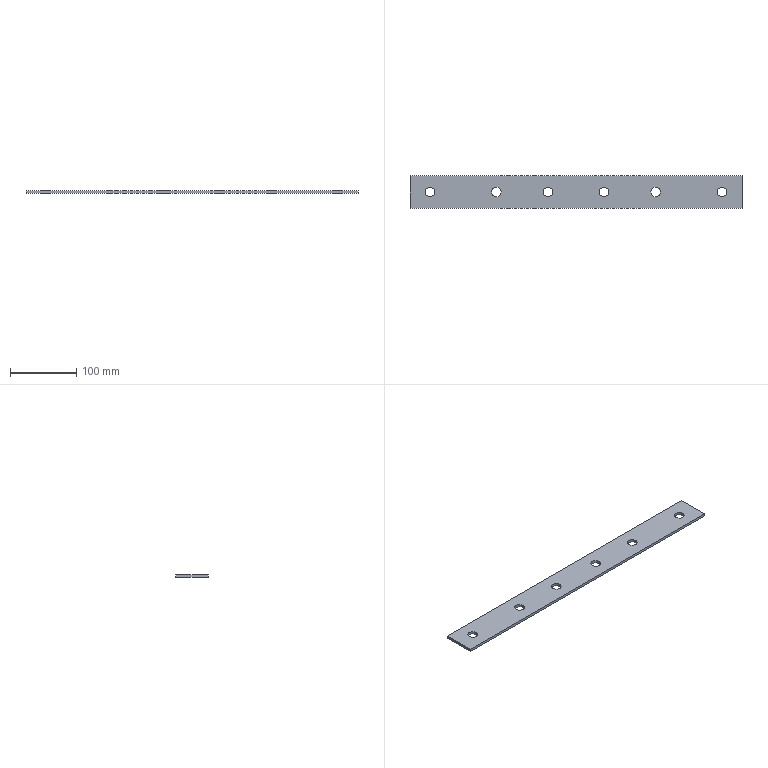Part | SolidWorks | features FlatPattern 1, ICE 1, MirrorPattern 1, SMBaseFlange 1, SheetMetal 1 | 1 solid | 18 faces | box 500 x 49 x 4 mm | volume 94037 mm3 | cylinder 12 | plane 6 | commonest cylinder face diameters 14.5 x12
STEP:
#1=CARTESIAN_POINT('',(-34.75,0.,-4.));
#2=VERTEX_POINT('',#1);
#3=CARTESIAN_POINT('',(-49.25,0.,-4.));
#4=VERTEX_POINT('',#3);
#5=CARTESIAN_POINT('',(-42.,0.,-4.));
#6=DIRECTION('',(0.,0.,-1.));
#7=DIRECTION('',(-1.,0.,0.));
#8=AXIS2_PLACEMENT_3D('',#5,#6,#7);
#9=CIRCLE('',#8,7.25);
#10=EDGE_CURVE('',#2,#4,#9,.T.);
#11=ORIENTED_EDGE('',*,*,#10,.T.);
#12=CARTESIAN_POINT('',(-49.25,0.,0.));
#13=VERTEX_POINT('',#12);
#14=CARTESIAN_POINT('',(-49.25,0.,-4.));
#15=DIRECTION('',(0.,0.,1.));
#16=VECTOR('',#15,1000.);
#17=LINE('',#14,#16);
#18=EDGE_CURVE('',#4,#13,#17,.T.);
#19=ORIENTED_EDGE('',*,*,#18,.T.);
#20=CARTESIAN_POINT('',(-34.75,0.,0.));
#21=VERTEX_POINT('',#20);
#22=CARTESIAN_POINT('',(-42.,0.,0.));
#23=DIRECTION('',(0.,0.,-1.));
#24=DIRECTION('',(1.,0.,0.));
#25=AXIS2_PLACEMENT_3D('',#22,#23,#24);
#26=CIRCLE('',#25,7.25);
#27=EDGE_CURVE('',#21,#13,#26,.T.);
#28=ORIENTED_EDGE('',*,*,#27,.F.);
#29=CARTESIAN_POINT('',(-34.75,0.,-4.));
#30=DIRECTION('',(0.,0.,1.));
#31=VECTOR('',#30,1000.);
#32=LINE('',#29,#31);
#33=EDGE_CURVE('',#2,#21,#32,.T.);
#34=ORIENTED_EDGE('',*,*,#33,.F.);
#35=EDGE_LOOP('',(#11,#19,#28,#34));
#36=FACE_OUTER_BOUND('',#35,.T.);
#37=CARTESIAN_POINT('',(-42.,0.,-4.));
#38=DIRECTION('',(0.,0.,1.));
#39=DIRECTION('',(1.,0.,0.));
#40=AXIS2_PLACEMENT_3D('',#37,#38,#39);
#41=CYLINDRICAL_SURFACE('',#40,7.25);
#42=ADVANCED_FACE('',(#36),#41,.F.);
#43=CARTESIAN_POINT('',(-112.75,0.,-4.));
#44=VERTEX_POINT('',#43);
#45=CARTESIAN_POINT('',(-127.25,0.,-4.));
#46=VERTEX_POINT('',#45);
#47=CARTESIAN_POINT('',(-120.,0.,-4.));
#48=DIRECTION('',(0.,0.,-1.));
#49=DIRECTION('',(-1.,0.,0.));
#50=AXIS2_PLACEMENT_3D('',#47,#48,#49);
#51=CIRCLE('',#50,7.25);
#52=EDGE_CURVE('',#44,#46,#51,.T.);
#53=ORIENTED_EDGE('',*,*,#52,.T.);
#54=CARTESIAN_POINT('',(-127.25,0.,0.));
#55=VERTEX_POINT('',#54);
#56=CARTESIAN_POINT('',(-127.25,0.,-4.));
#57=DIRECTION('',(0.,0.,1.));
#58=VECTOR('',#57,1000.);
#59=LINE('',#56,#58);
#60=EDGE_CURVE('',#46,#55,#59,.T.);
#61=ORIENTED_EDGE('',*,*,#60,.T.);
#62=CARTESIAN_POINT('',(-112.75,0.,0.));
#63=VERTEX_POINT('',#62);
#64=CARTESIAN_POINT('',(-120.,0.,0.));
#65=DIRECTION('',(0.,0.,-1.));
#66=DIRECTION('',(1.,0.,0.));
#67=AXIS2_PLACEMENT_3D('',#64,#65,#66);
#68=CIRCLE('',#67,7.25);
#69=EDGE_CURVE('',#63,#55,#68,.T.);
#70=ORIENTED_EDGE('',*,*,#69,.F.);
#71=CARTESIAN_POINT('',(-112.75,0.,-4.));
#72=DIRECTION('',(0.,0.,1.));
#73=VECTOR('',#72,1000.);
#74=LINE('',#71,#73);
#75=EDGE_CURVE('',#44,#63,#74,.T.);
#76=ORIENTED_EDGE('',*,*,#75,.F.);
#77=EDGE_LOOP('',(#53,#61,#70,#76));
#78=FACE_OUTER_BOUND('',#77,.T.);
#79=CARTESIAN_POINT('',(-120.,0.,-4.));
#80=DIRECTION('',(0.,0.,1.));
#81=DIRECTION('',(1.,0.,0.));
#82=AXIS2_PLACEMENT_3D('',#79,#80,#81);
#83=CYLINDRICAL_SURFACE('',#82,7.25);
#84=ADVANCED_FACE('',(#78),#83,.F.);
#85=CARTESIAN_POINT('',(-212.75,0.,-4.));
#86=VERTEX_POINT('',#85);
#87=CARTESIAN_POINT('',(-227.25,0.,-4.));
#88=VERTEX_POINT('',#87);
#89=CARTESIAN_POINT('',(-220.,0.,-4.));
#90=DIRECTION('',(0.,0.,-1.));
#91=DIRECTION('',(-1.,0.,0.));
#92=AXIS2_PLACEMENT_3D('',#89,#90,#91);
#93=CIRCLE('',#92,7.25);
#94=EDGE_CURVE('',#86,#88,#93,.T.);
#95=ORIENTED_EDGE('',*,*,#94,.T.);
#96=CARTESIAN_POINT('',(-227.25,0.,0.));
#97=VERTEX_POINT('',#96);
#98=CARTESIAN_POINT('',(-227.25,0.,-4.));
#99=DIRECTION('',(0.,0.,1.));
#100=VECTOR('',#99,1000.);
#101=LINE('',#98,#100);
#102=EDGE_CURVE('',#88,#97,#101,.T.);
#103=ORIENTED_EDGE('',*,*,#102,.T.);
#104=CARTESIAN_POINT('',(-212.75,0.,0.));
#105=VERTEX_POINT('',#104);
#106=CARTESIAN_POINT('',(-220.,0.,0.));
#107=DIRECTION('',(0.,0.,-1.));
#108=DIRECTION('',(1.,0.,0.));
#109=AXIS2_PLACEMENT_3D('',#106,#107,#108);
#110=CIRCLE('',#109,7.25);
#111=EDGE_CURVE('',#105,#97,#110,.T.);
#112=ORIENTED_EDGE('',*,*,#111,.F.);
#113=CARTESIAN_POINT('',(-212.75,0.,-4.));
#114=DIRECTION('',(0.,0.,1.));
#115=VECTOR('',#114,1000.);
#116=LINE('',#113,#115);
#117=EDGE_CURVE('',#86,#105,#116,.T.);
#118=ORIENTED_EDGE('',*,*,#117,.F.);
#119=EDGE_LOOP('',(#95,#103,#112,#118));
#120=FACE_OUTER_BOUND('',#119,.T.);
#121=CARTESIAN_POINT('',(-220.,0.,-4.));
#122=DIRECTION('',(0.,0.,1.));
#123=DIRECTION('',(1.,0.,0.));
#124=AXIS2_PLACEMENT_3D('',#121,#122,#123);
#125=CYLINDRICAL_SURFACE('',#124,7.25);
#126=ADVANCED_FACE('',(#120),#125,.F.);
#127=CARTESIAN_POINT('',(34.75,0.,-4.));
#128=VERTEX_POINT('',#127);
#129=CARTESIAN_POINT('',(49.25,0.,-4.));
#130=VERTEX_POINT('',#129);
#131=CARTESIAN_POINT('',(42.,0.,-4.));
#132=DIRECTION('',(0.,0.,1.));
#133=DIRECTION('',(1.,0.,0.));
#134=AXIS2_PLACEMENT_3D('',#131,#132,#133);
#135=CIRCLE('',#134,7.25);
#136=EDGE_CURVE('',#128,#130,#135,.T.);
#137=ORIENTED_EDGE('',*,*,#136,.F.);
#138=CARTESIAN_POINT('',(34.75,0.,0.));
#139=VERTEX_POINT('',#138);
#140=CARTESIAN_POINT('',(34.75,0.,-4.));
#141=DIRECTION('',(0.,0.,1.));
#142=VECTOR('',#141,1000.);
#143=LINE('',#140,#142);
#144=EDGE_CURVE('',#128,#139,#143,.T.);
#145=ORIENTED_EDGE('',*,*,#144,.T.);
#146=CARTESIAN_POINT('',(49.25,0.,0.));
#147=VERTEX_POINT('',#146);
#148=CARTESIAN_POINT('',(42.,0.,0.));
#149=DIRECTION('',(0.,0.,1.));
#150=DIRECTION('',(1.,0.,0.));
#151=AXIS2_PLACEMENT_3D('',#148,#149,#150);
#152=CIRCLE('',#151,7.25);
#153=EDGE_CURVE('',#139,#147,#152,.T.);
#154=ORIENTED_EDGE('',*,*,#153,.T.);
#155=CARTESIAN_POINT('',(49.25,0.,-4.));
#156=DIRECTION('',(0.,0.,1.));
#157=VECTOR('',#156,1000.);
#158=LINE('',#155,#157);
#159=EDGE_CURVE('',#130,#147,#158,.T.);
#160=ORIENTED_EDGE('',*,*,#159,.F.);
#161=EDGE_LOOP('',(#137,#145,#154,#160));
#162=FACE_OUTER_BOUND('',#161,.T.);
#163=CARTESIAN_POINT('',(42.,0.,-4.));
#164=DIRECTION('',(0.,0.,1.));
#165=DIRECTION('',(1.,0.,0.));
#166=AXIS2_PLACEMENT_3D('',#163,#164,#165);
#167=CYLINDRICAL_SURFACE('',#166,7.25);
#168=ADVANCED_FACE('',(#162),#167,.F.);
#169=CARTESIAN_POINT('',(112.75,0.,-4.));
#170=VERTEX_POINT('',#169);
#171=CARTESIAN_POINT('',(127.25,0.,-4.));
#172=VERTEX_POINT('',#171);
#173=CARTESIAN_POINT('',(120.,0.,-4.));
#174=DIRECTION('',(0.,0.,1.));
#175=DIRECTION('',(1.,0.,0.));
#176=AXIS2_PLACEMENT_3D('',#173,#174,#175);
#177=CIRCLE('',#176,7.25);
#178=EDGE_CURVE('',#170,#172,#177,.T.);
#179=ORIENTED_EDGE('',*,*,#178,.F.);
#180=CARTESIAN_POINT('',(112.75,0.,0.));
#181=VERTEX_POINT('',#180);
#182=CARTESIAN_POINT('',(112.75,0.,-4.));
#183=DIRECTION('',(0.,0.,1.));
#184=VECTOR('',#183,1000.);
#185=LINE('',#182,#184);
#186=EDGE_CURVE('',#170,#181,#185,.T.);
#187=ORIENTED_EDGE('',*,*,#186,.T.);
#188=CARTESIAN_POINT('',(127.25,0.,0.));
#189=VERTEX_POINT('',#188);
#190=CARTESIAN_POINT('',(120.,0.,0.));
#191=DIRECTION('',(0.,0.,1.));
#192=DIRECTION('',(1.,0.,0.));
#193=AXIS2_PLACEMENT_3D('',#190,#191,#192);
#194=CIRCLE('',#193,7.25);
#195=EDGE_CURVE('',#181,#189,#194,.T.);
#196=ORIENTED_EDGE('',*,*,#195,.T.);
#197=CARTESIAN_POINT('',(127.25,0.,-4.));
#198=DIRECTION('',(0.,0.,1.));
#199=VECTOR('',#198,1000.);
#200=LINE('',#197,#199);
#201=EDGE_CURVE('',#172,#189,#200,.T.);
#202=ORIENTED_EDGE('',*,*,#201,.F.);
#203=EDGE_LOOP('',(#179,#187,#196,#202));
#204=FACE_OUTER_BOUND('',#203,.T.);
#205=CARTESIAN_POINT('',(120.,0.,-4.));
#206=DIRECTION('',(0.,0.,1.));
#207=DIRECTION('',(1.,0.,0.));
#208=AXIS2_PLACEMENT_3D('',#205,#206,#207);
#209=CYLINDRICAL_SURFACE('',#208,7.25);
#210=ADVANCED_FACE('',(#204),#209,.F.);
#211=CARTESIAN_POINT('',(212.75,0.,-4.));
#212=VERTEX_POINT('',#211);
#213=CARTESIAN_POINT('',(227.25,0.,-4.));
#214=VERTEX_POINT('',#213);
#215=CARTESIAN_POINT('',(220.,0.,-4.));
#216=DIRECTION('',(0.,0.,1.));
#217=DIRECTION('',(1.,0.,0.));
#218=AXIS2_PLACEMENT_3D('',#215,#216,#217);
#219=CIRCLE('',#218,7.25);
#220=EDGE_CURVE('',#212,#214,#219,.T.);
#221=ORIENTED_EDGE('',*,*,#220,.F.);
#222=CARTESIAN_POINT('',(212.75,0.,0.));
#223=VERTEX_POINT('',#222);
#224=CARTESIAN_POINT('',(212.75,0.,-4.));
#225=DIRECTION('',(0.,0.,1.));
#226=VECTOR('',#225,1000.);
#227=LINE('',#224,#226);
#228=EDGE_CURVE('',#212,#223,#227,.T.);
#229=ORIENTED_EDGE('',*,*,#228,.T.);
#230=CARTESIAN_POINT('',(227.25,0.,0.));
#231=VERTEX_POINT('',#230);
#232=CARTESIAN_POINT('',(220.,0.,0.));
#233=DIRECTION('',(0.,0.,1.));
#234=DIRECTION('',(1.,0.,0.));
#235=AXIS2_PLACEMENT_3D('',#232,#233,#234);
#236=CIRCLE('',#235,7.25);
#237=EDGE_CURVE('',#223,#231,#236,.T.);
#238=ORIENTED_EDGE('',*,*,#237,.T.);
#239=CARTESIAN_POINT('',(227.25,0.,-4.));
#240=DIRECTION('',(0.,0.,1.));
#241=VECTOR('',#240,1000.);
#242=LINE('',#239,#241);
#243=EDGE_CURVE('',#214,#231,#242,.T.);
#244=ORIENTED_EDGE('',*,*,#243,.F.);
#245=EDGE_LOOP('',(#221,#229,#238,#244));
#246=FACE_OUTER_BOUND('',#245,.T.);
#247=CARTESIAN_POINT('',(220.,0.,-4.));
#248=DIRECTION('',(0.,0.,1.));
#249=DIRECTION('',(1.,0.,0.));
#250=AXIS2_PLACEMENT_3D('',#247,#248,#249);
#251=CYLINDRICAL_SURFACE('',#250,7.25);
#252=ADVANCED_FACE('',(#246),#251,.F.);
#253=CARTESIAN_POINT('',(250.,-24.5,0.));
#254=VERTEX_POINT('',#253);
#255=CARTESIAN_POINT('',(250.,24.5,0.));
#256=VERTEX_POINT('',#255);
#257=CARTESIAN_POINT('',(250.,24.5,0.));
#258=DIRECTION('',(0.,1.,0.));
#259=VECTOR('',#258,1000.);
#260=LINE('',#257,#259);
#261=EDGE_CURVE('',#254,#256,#260,.T.);
#262=ORIENTED_EDGE('',*,*,#261,.F.);
#263=CARTESIAN_POINT('',(250.,-24.5,-4.));
#264=VERTEX_POINT('',#263);
#265=CARTESIAN_POINT('',(250.,-24.5,-4.));
#266=DIRECTION('',(0.,0.,1.));
#267=VECTOR('',#266,1000.);
#268=LINE('',#265,#267);
#269=EDGE_CURVE('',#264,#254,#268,.T.);
#270=ORIENTED_EDGE('',*,*,#269,.F.);
#271=CARTESIAN_POINT('',(250.,24.5,-4.));
#272=VERTEX_POINT('',#271);
#273=CARTESIAN_POINT('',(250.,24.5,-4.));
#274=DIRECTION('',(0.,1.,0.));
#275=VECTOR('',#274,1000.);
#276=LINE('',#273,#275);
#277=EDGE_CURVE('',#264,#272,#276,.T.);
#278=ORIENTED_EDGE('',*,*,#277,.T.);
#279=CARTESIAN_POINT('',(250.,24.5,-4.));
#280=DIRECTION('',(0.,0.,1.));
#281=VECTOR('',#280,1000.);
#282=LINE('',#279,#281);
#283=EDGE_CURVE('',#272,#256,#282,.T.);
#284=ORIENTED_EDGE('',*,*,#283,.T.);
#285=EDGE_LOOP('',(#262,#270,#278,#284));
#286=FACE_OUTER_BOUND('',#285,.T.);
#287=CARTESIAN_POINT('',(250.,24.5,-4.));
#288=DIRECTION('',(1.,0.,0.));
#289=DIRECTION('',(0.,0.,-1.));
#290=AXIS2_PLACEMENT_3D('',#287,#288,#289);
#291=PLANE('',#290);
#292=ADVANCED_FACE('',(#286),#291,.T.);
#293=CARTESIAN_POINT('',(-250.,-24.5,0.));
#294=VERTEX_POINT('',#293);
#295=CARTESIAN_POINT('',(-250.,-24.5,0.));
#296=DIRECTION('',(1.,0.,0.));
#297=VECTOR('',#296,1000.);
#298=LINE('',#295,#297);
#299=EDGE_CURVE('',#294,#254,#298,.T.);
#300=ORIENTED_EDGE('',*,*,#299,.F.);
#301=CARTESIAN_POINT('',(-250.,-24.5,-4.));
#302=VERTEX_POINT('',#301);
#303=CARTESIAN_POINT('',(-250.,-24.5,-4.));
#304=DIRECTION('',(0.,0.,1.));
#305=VECTOR('',#304,1000.);
#306=LINE('',#303,#305);
#307=EDGE_CURVE('',#302,#294,#306,.T.);
#308=ORIENTED_EDGE('',*,*,#307,.F.);
#309=CARTESIAN_POINT('',(-250.,-24.5,-4.));
#310=DIRECTION('',(1.,0.,0.));
#311=VECTOR('',#310,1000.);
#312=LINE('',#309,#311);
#313=EDGE_CURVE('',#302,#264,#312,.T.);
#314=ORIENTED_EDGE('',*,*,#313,.T.);
#315=ORIENTED_EDGE('',*,*,#269,.T.);
#316=EDGE_LOOP('',(#300,#308,#314,#315));
#317=FACE_OUTER_BOUND('',#316,.T.);
#318=CARTESIAN_POINT('',(-250.,-24.5,-4.));
#319=DIRECTION('',(0.,-1.,0.));
#320=DIRECTION('',(0.,0.,-1.));
#321=AXIS2_PLACEMENT_3D('',#318,#319,#320);
#322=PLANE('',#321);
#323=ADVANCED_FACE('',(#317),#322,.T.);
#324=CARTESIAN_POINT('',(-250.,24.5,0.));
#325=VERTEX_POINT('',#324);
#326=CARTESIAN_POINT('',(-250.,24.5,0.));
#327=DIRECTION('',(0.,-1.,0.));
#328=VECTOR('',#327,1000.);
#329=LINE('',#326,#328);
#330=EDGE_CURVE('',#325,#294,#329,.T.);
#331=ORIENTED_EDGE('',*,*,#330,.F.);
#332=CARTESIAN_POINT('',(-250.,24.5,-4.));
#333=VERTEX_POINT('',#332);
#334=CARTESIAN_POINT('',(-250.,24.5,-4.));
#335=DIRECTION('',(0.,0.,1.));
#336=VECTOR('',#335,1000.);
#337=LINE('',#334,#336);
#338=EDGE_CURVE('',#333,#325,#337,.T.);
#339=ORIENTED_EDGE('',*,*,#338,.F.);
#340=CARTESIAN_POINT('',(-250.,24.5,-4.));
#341=DIRECTION('',(0.,-1.,0.));
#342=VECTOR('',#341,1000.);
#343=LINE('',#340,#342);
#344=EDGE_CURVE('',#333,#302,#343,.T.);
#345=ORIENTED_EDGE('',*,*,#344,.T.);
#346=ORIENTED_EDGE('',*,*,#307,.T.);
#347=EDGE_LOOP('',(#331,#339,#345,#346));
#348=FACE_OUTER_BOUND('',#347,.T.);
#349=CARTESIAN_POINT('',(-250.,24.5,-4.));
#350=DIRECTION('',(-1.,0.,0.));
#351=DIRECTION('',(0.,0.,1.));
#352=AXIS2_PLACEMENT_3D('',#349,#350,#351);
#353=PLANE('',#352);
#354=ADVANCED_FACE('',(#348),#353,.T.);
#355=CARTESIAN_POINT('',(-250.,24.5,0.));
#356=DIRECTION('',(-1.,0.,0.));
#357=VECTOR('',#356,1000.);
#358=LINE('',#355,#357);
#359=EDGE_CURVE('',#256,#325,#358,.T.);
#360=ORIENTED_EDGE('',*,*,#359,.F.);
#361=ORIENTED_EDGE('',*,*,#283,.F.);
#362=CARTESIAN_POINT('',(-250.,24.5,-4.));
#363=DIRECTION('',(-1.,0.,0.));
#364=VECTOR('',#363,1000.);
#365=LINE('',#362,#364);
#366=EDGE_CURVE('',#272,#333,#365,.T.);
#367=ORIENTED_EDGE('',*,*,#366,.T.);
#368=ORIENTED_EDGE('',*,*,#338,.T.);
#369=EDGE_LOOP('',(#360,#361,#367,#368));
#370=FACE_OUTER_BOUND('',#369,.T.);
#371=CARTESIAN_POINT('',(-250.,24.5,-4.));
#372=DIRECTION('',(0.,1.,0.));
#373=DIRECTION('',(0.,0.,1.));
#374=AXIS2_PLACEMENT_3D('',#371,#372,#373);
#375=PLANE('',#374);
#376=ADVANCED_FACE('',(#370),#375,.T.);
#377=ORIENTED_EDGE('',*,*,#10,.F.);
#378=CARTESIAN_POINT('',(-42.,0.,-4.));
#379=DIRECTION('',(0.,0.,-1.));
#380=DIRECTION('',(-1.,0.,0.));
#381=AXIS2_PLACEMENT_3D('',#378,#379,#380);
#382=CIRCLE('',#381,7.25);
#383=EDGE_CURVE('',#4,#2,#382,.T.);
#384=ORIENTED_EDGE('',*,*,#383,.F.);
#385=EDGE_LOOP('',(#377,#384));
#386=FACE_BOUND('',#385,.T.);
#387=ORIENTED_EDGE('',*,*,#52,.F.);
#388=CARTESIAN_POINT('',(-120.,0.,-4.));
#389=DIRECTION('',(0.,0.,-1.));
#390=DIRECTION('',(-1.,0.,0.));
#391=AXIS2_PLACEMENT_3D('',#388,#389,#390);
#392=CIRCLE('',#391,7.25);
#393=EDGE_CURVE('',#46,#44,#392,.T.);
#394=ORIENTED_EDGE('',*,*,#393,.F.);
#395=EDGE_LOOP('',(#387,#394));
#396=FACE_BOUND('',#395,.T.);
#397=ORIENTED_EDGE('',*,*,#94,.F.);
#398=CARTESIAN_POINT('',(-220.,0.,-4.));
#399=DIRECTION('',(0.,0.,-1.));
#400=DIRECTION('',(-1.,0.,0.));
#401=AXIS2_PLACEMENT_3D('',#398,#399,#400);
#402=CIRCLE('',#401,7.25);
#403=EDGE_CURVE('',#88,#86,#402,.T.);
#404=ORIENTED_EDGE('',*,*,#403,.F.);
#405=EDGE_LOOP('',(#397,#404));
#406=FACE_BOUND('',#405,.T.);
#407=CARTESIAN_POINT('',(42.,0.,-4.));
#408=DIRECTION('',(0.,0.,1.));
#409=DIRECTION('',(1.,0.,0.));
#410=AXIS2_PLACEMENT_3D('',#407,#408,#409);
#411=CIRCLE('',#410,7.25);
#412=EDGE_CURVE('',#130,#128,#411,.T.);
#413=ORIENTED_EDGE('',*,*,#412,.T.);
#414=ORIENTED_EDGE('',*,*,#136,.T.);
#415=EDGE_LOOP('',(#413,#414));
#416=FACE_BOUND('',#415,.T.);
#417=CARTESIAN_POINT('',(120.,0.,-4.));
#418=DIRECTION('',(0.,0.,1.));
#419=DIRECTION('',(1.,0.,0.));
#420=AXIS2_PLACEMENT_3D('',#417,#418,#419);
#421=CIRCLE('',#420,7.25);
#422=EDGE_CURVE('',#172,#170,#421,.T.);
#423=ORIENTED_EDGE('',*,*,#422,.T.);
#424=ORIENTED_EDGE('',*,*,#178,.T.);
#425=EDGE_LOOP('',(#423,#424));
#426=FACE_BOUND('',#425,.T.);
#427=CARTESIAN_POINT('',(220.,0.,-4.));
#428=DIRECTION('',(0.,0.,1.));
#429=DIRECTION('',(1.,0.,0.));
#430=AXIS2_PLACEMENT_3D('',#427,#428,#429);
#431=CIRCLE('',#430,7.25);
#432=EDGE_CURVE('',#214,#212,#431,.T.);
#433=ORIENTED_EDGE('',*,*,#432,.T.);
#434=ORIENTED_EDGE('',*,*,#220,.T.);
#435=EDGE_LOOP('',(#433,#434));
#436=FACE_BOUND('',#435,.T.);
#437=ORIENTED_EDGE('',*,*,#277,.F.);
#438=ORIENTED_EDGE('',*,*,#313,.F.);
#439=ORIENTED_EDGE('',*,*,#344,.F.);
#440=ORIENTED_EDGE('',*,*,#366,.F.);
#441=EDGE_LOOP('',(#437,#438,#439,#440));
#442=FACE_OUTER_BOUND('',#441,.T.);
#443=CARTESIAN_POINT('',(0.,0.,-4.));
#444=DIRECTION('',(0.,0.,1.));
#445=DIRECTION('',(1.,0.,0.));
#446=AXIS2_PLACEMENT_3D('',#443,#444,#445);
#447=PLANE('',#446);
#448=ADVANCED_FACE('',(#386,#396,#406,#416,#426,#436,#442),#447,.F.);
#449=ORIENTED_EDGE('',*,*,#27,.T.);
#450=CARTESIAN_POINT('',(-42.,0.,0.));
#451=DIRECTION('',(0.,0.,-1.));
#452=DIRECTION('',(1.,0.,0.));
#453=AXIS2_PLACEMENT_3D('',#450,#451,#452);
#454=CIRCLE('',#453,7.25);
#455=EDGE_CURVE('',#13,#21,#454,.T.);
#456=ORIENTED_EDGE('',*,*,#455,.T.);
#457=EDGE_LOOP('',(#449,#456));
#458=FACE_BOUND('',#457,.T.);
#459=ORIENTED_EDGE('',*,*,#69,.T.);
#460=CARTESIAN_POINT('',(-120.,0.,0.));
#461=DIRECTION('',(0.,0.,-1.));
#462=DIRECTION('',(1.,0.,0.));
#463=AXIS2_PLACEMENT_3D('',#460,#461,#462);
#464=CIRCLE('',#463,7.25);
#465=EDGE_CURVE('',#55,#63,#464,.T.);
#466=ORIENTED_EDGE('',*,*,#465,.T.);
#467=EDGE_LOOP('',(#459,#466));
#468=FACE_BOUND('',#467,.T.);
#469=ORIENTED_EDGE('',*,*,#111,.T.);
#470=CARTESIAN_POINT('',(-220.,0.,0.));
#471=DIRECTION('',(0.,0.,-1.));
#472=DIRECTION('',(1.,0.,0.));
#473=AXIS2_PLACEMENT_3D('',#470,#471,#472);
#474=CIRCLE('',#473,7.25);
#475=EDGE_CURVE('',#97,#105,#474,.T.);
#476=ORIENTED_EDGE('',*,*,#475,.T.);
#477=EDGE_LOOP('',(#469,#476));
#478=FACE_BOUND('',#477,.T.);
#479=CARTESIAN_POINT('',(42.,0.,0.));
#480=DIRECTION('',(0.,0.,1.));
#481=DIRECTION('',(1.,0.,0.));
#482=AXIS2_PLACEMENT_3D('',#479,#480,#481);
#483=CIRCLE('',#482,7.25);
#484=EDGE_CURVE('',#147,#139,#483,.T.);
#485=ORIENTED_EDGE('',*,*,#484,.F.);
#486=ORIENTED_EDGE('',*,*,#153,.F.);
#487=EDGE_LOOP('',(#485,#486));
#488=FACE_BOUND('',#487,.T.);
#489=CARTESIAN_POINT('',(120.,0.,0.));
#490=DIRECTION('',(0.,0.,1.));
#491=DIRECTION('',(1.,0.,0.));
#492=AXIS2_PLACEMENT_3D('',#489,#490,#491);
#493=CIRCLE('',#492,7.25);
#494=EDGE_CURVE('',#189,#181,#493,.T.);
#495=ORIENTED_EDGE('',*,*,#494,.F.);
#496=ORIENTED_EDGE('',*,*,#195,.F.);
#497=EDGE_LOOP('',(#495,#496));
#498=FACE_BOUND('',#497,.T.);
#499=CARTESIAN_POINT('',(220.,0.,0.));
#500=DIRECTION('',(0.,0.,1.));
#501=DIRECTION('',(1.,0.,0.));
#502=AXIS2_PLACEMENT_3D('',#499,#500,#501);
#503=CIRCLE('',#502,7.25);
#504=EDGE_CURVE('',#231,#223,#503,.T.);
#505=ORIENTED_EDGE('',*,*,#504,.F.);
#506=ORIENTED_EDGE('',*,*,#237,.F.);
#507=EDGE_LOOP('',(#505,#506));
#508=FACE_BOUND('',#507,.T.);
#509=ORIENTED_EDGE('',*,*,#261,.T.);
#510=ORIENTED_EDGE('',*,*,#359,.T.);
#511=ORIENTED_EDGE('',*,*,#330,.T.);
#512=ORIENTED_EDGE('',*,*,#299,.T.);
#513=EDGE_LOOP('',(#509,#510,#511,#512));
#514=FACE_OUTER_BOUND('',#513,.T.);
#515=CARTESIAN_POINT('',(0.,0.,0.));
#516=DIRECTION('',(0.,0.,1.));
#517=DIRECTION('',(1.,0.,0.));
#518=AXIS2_PLACEMENT_3D('',#515,#516,#517);
#519=PLANE('',#518);
#520=ADVANCED_FACE('',(#458,#468,#478,#488,#498,#508,#514),#519,.T.);
#521=ORIENTED_EDGE('',*,*,#228,.F.);
#522=ORIENTED_EDGE('',*,*,#432,.F.);
#523=ORIENTED_EDGE('',*,*,#243,.T.);
#524=ORIENTED_EDGE('',*,*,#504,.T.);
#525=EDGE_LOOP('',(#521,#522,#523,#524));
#526=FACE_OUTER_BOUND('',#525,.T.);
#527=CARTESIAN_POINT('',(220.,0.,-4.));
#528=DIRECTION('',(0.,0.,1.));
#529=DIRECTION('',(1.,0.,0.));
#530=AXIS2_PLACEMENT_3D('',#527,#528,#529);
#531=CYLINDRICAL_SURFACE('',#530,7.25);
#532=ADVANCED_FACE('',(#526),#531,.F.);
#533=ORIENTED_EDGE('',*,*,#186,.F.);
#534=ORIENTED_EDGE('',*,*,#422,.F.);
#535=ORIENTED_EDGE('',*,*,#201,.T.);
#536=ORIENTED_EDGE('',*,*,#494,.T.);
#537=EDGE_LOOP('',(#533,#534,#535,#536));
#538=FACE_OUTER_BOUND('',#537,.T.);
#539=CARTESIAN_POINT('',(120.,0.,-4.));
#540=DIRECTION('',(0.,0.,1.));
#541=DIRECTION('',(1.,0.,0.));
#542=AXIS2_PLACEMENT_3D('',#539,#540,#541);
#543=CYLINDRICAL_SURFACE('',#542,7.25);
#544=ADVANCED_FACE('',(#538),#543,.F.);
#545=ORIENTED_EDGE('',*,*,#144,.F.);
#546=ORIENTED_EDGE('',*,*,#412,.F.);
#547=ORIENTED_EDGE('',*,*,#159,.T.);
#548=ORIENTED_EDGE('',*,*,#484,.T.);
#549=EDGE_LOOP('',(#545,#546,#547,#548));
#550=FACE_OUTER_BOUND('',#549,.T.);
#551=CARTESIAN_POINT('',(42.,0.,-4.));
#552=DIRECTION('',(0.,0.,1.));
#553=DIRECTION('',(1.,0.,0.));
#554=AXIS2_PLACEMENT_3D('',#551,#552,#553);
#555=CYLINDRICAL_SURFACE('',#554,7.25);
#556=ADVANCED_FACE('',(#550),#555,.F.);
#557=ORIENTED_EDGE('',*,*,#102,.F.);
#558=ORIENTED_EDGE('',*,*,#403,.T.);
#559=ORIENTED_EDGE('',*,*,#117,.T.);
#560=ORIENTED_EDGE('',*,*,#475,.F.);
#561=EDGE_LOOP('',(#557,#558,#559,#560));
#562=FACE_OUTER_BOUND('',#561,.T.);
#563=CARTESIAN_POINT('',(-220.,0.,-4.));
#564=DIRECTION('',(0.,0.,1.));
#565=DIRECTION('',(1.,0.,0.));
#566=AXIS2_PLACEMENT_3D('',#563,#564,#565);
#567=CYLINDRICAL_SURFACE('',#566,7.25);
#568=ADVANCED_FACE('',(#562),#567,.F.);
#569=ORIENTED_EDGE('',*,*,#60,.F.);
#570=ORIENTED_EDGE('',*,*,#393,.T.);
#571=ORIENTED_EDGE('',*,*,#75,.T.);
#572=ORIENTED_EDGE('',*,*,#465,.F.);
#573=EDGE_LOOP('',(#569,#570,#571,#572));
#574=FACE_OUTER_BOUND('',#573,.T.);
#575=CARTESIAN_POINT('',(-120.,0.,-4.));
#576=DIRECTION('',(0.,0.,1.));
#577=DIRECTION('',(1.,0.,0.));
#578=AXIS2_PLACEMENT_3D('',#575,#576,#577);
#579=CYLINDRICAL_SURFACE('',#578,7.25);
#580=ADVANCED_FACE('',(#574),#579,.F.);
#581=ORIENTED_EDGE('',*,*,#18,.F.);
#582=ORIENTED_EDGE('',*,*,#383,.T.);
#583=ORIENTED_EDGE('',*,*,#33,.T.);
#584=ORIENTED_EDGE('',*,*,#455,.F.);
#585=EDGE_LOOP('',(#581,#582,#583,#584));
#586=FACE_OUTER_BOUND('',#585,.T.);
#587=CARTESIAN_POINT('',(-42.,0.,-4.));
#588=DIRECTION('',(0.,0.,1.));
#589=DIRECTION('',(1.,0.,0.));
#590=AXIS2_PLACEMENT_3D('',#587,#588,#589);
#591=CYLINDRICAL_SURFACE('',#590,7.25);
#592=ADVANCED_FACE('',(#586),#591,.F.);
#593=CLOSED_SHELL('',(#42,#84,#126,#168,#210,#252,#292,#323,#354,#376,#448,#520,#532,#544,#556,#568,#580,#592));
#594=MANIFOLD_SOLID_BREP('',#593);
#595=CARTESIAN_POINT('',(0.,0.,0.));
#596=DIRECTION('',(0.,0.,1.));
#597=DIRECTION('',(1.,0.,0.));
#598=AXIS2_PLACEMENT_3D('',#595,#596,#597);
#599=(LENGTH_UNIT()NAMED_UNIT(*)SI_UNIT(.MILLI.,.METRE.));
#600=UNCERTAINTY_MEASURE_WITH_UNIT(LENGTH_MEASURE(0.00001),#599,'','');
#601=(NAMED_UNIT(*)PLANE_ANGLE_UNIT()SI_UNIT($,.RADIAN.));
#602=(NAMED_UNIT(*)SI_UNIT($,.STERADIAN.)SOLID_ANGLE_UNIT());
#603=(GEOMETRIC_REPRESENTATION_CONTEXT(3)GLOBAL_UNCERTAINTY_ASSIGNED_CONTEXT((#600))GLOBAL_UNIT_ASSIGNED_CONTEXT((#599,#601,#602))REPRESENTATION_CONTEXT('',''));
#604=ADVANCED_BREP_SHAPE_REPRESENTATION('',(#594,#598),#603);